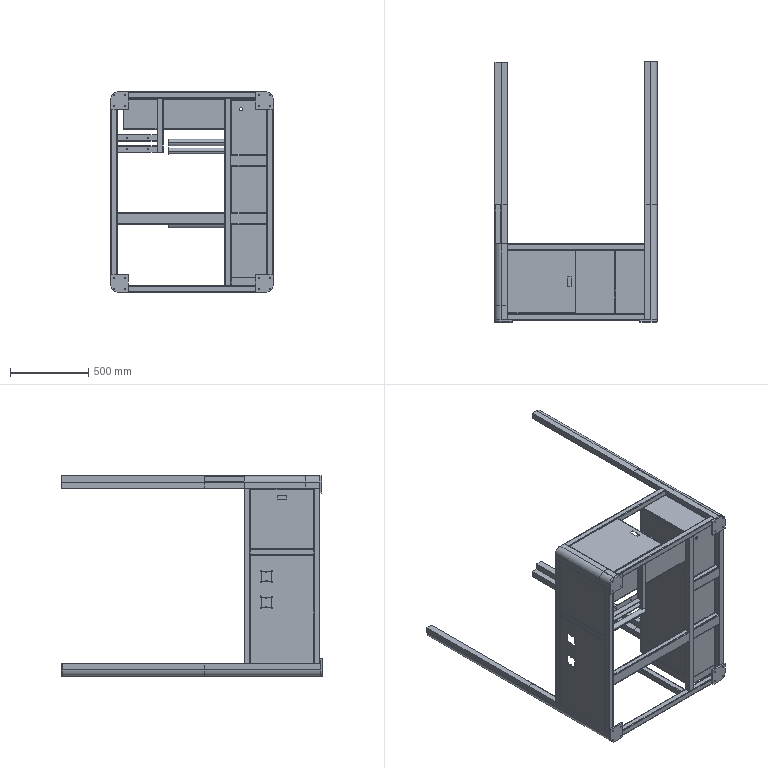Part | 47 solids | 864 faces | box 1036 x 1664 x 1280 mm | volume 26350610 mm3 | plane 483 | cylinder 342 | spline 39 | commonest cylinder face diameters 8 x46 9 x41 3.3 x40 7 x32 12 x20 2 x16